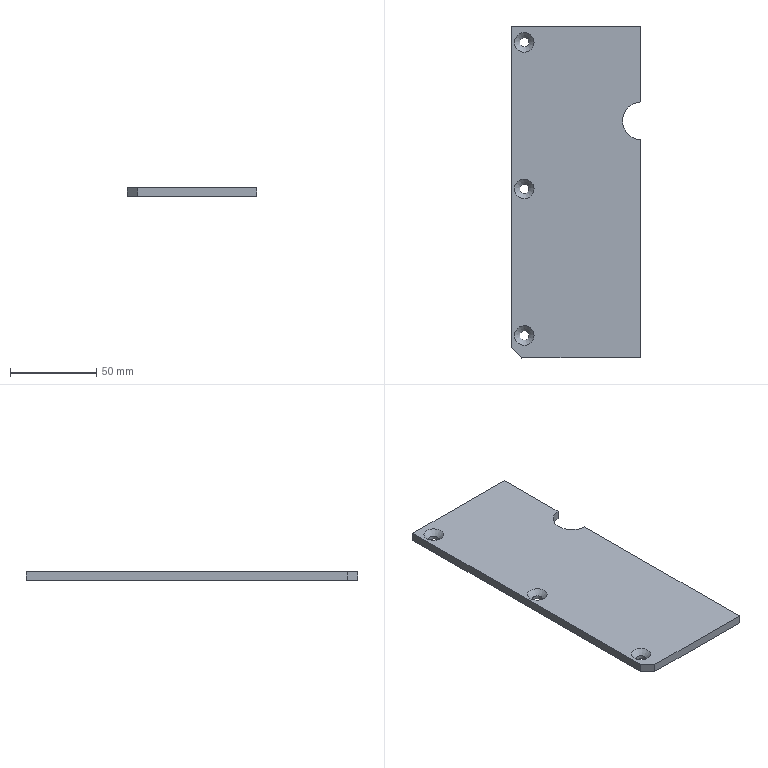Part | STEP file | P011002NF05-000 | 1 solid | 15 faces | box 75 x 192.5 x 5 mm | volume 70540 mm3 | plane 8 | cylinder 4 | cone 3 | commonest cylinder face diameters 5.5 x3 22 x1
STEP:
#1=CARTESIAN_POINT('',(0.,0.,0.));
#2=DIRECTION('',(0.,0.,1.));
#3=DIRECTION('',(1.,0.,0.));
#4=AXIS2_PLACEMENT_3D('',#1,#2,#3);
#5=CARTESIAN_POINT('',(-200.,233.25,265.5));
#6=VERTEX_POINT('',#5);
#7=CARTESIAN_POINT('',(-200.,230.5,265.5));
#8=DIRECTION('',(0.,0.,1.));
#9=DIRECTION('',(0.,1.,0.));
#10=AXIS2_PLACEMENT_3D('',#7,#8,#9);
#11=CIRCLE('',#10,2.75);
#12=CARTESIAN_POINT('',(-80.,170.,265.5));
#13=DIRECTION('',(0.,0.,-1.));
#14=DIRECTION('',(-1.,0.,0.));
#15=AXIS2_PLACEMENT_3D('',#12,#13,#14);
#16=PLANE('',#15);
#17=CARTESIAN_POINT('',(120.,63.25));
#18=CARTESIAN_POINT('',(124.763,63.25));
#19=CARTESIAN_POINT('',(122.382,59.125));
#20=CARTESIAN_POINT('',(120.,55.));
#21=CARTESIAN_POINT('',(117.618,59.125));
#22=CARTESIAN_POINT('',(115.237,63.25));
#23=CARTESIAN_POINT('',(120.,63.25));
#24=(BOUNDED_CURVE()B_SPLINE_CURVE(2,(#17,#18,#19,#20,#21,#22,#23),.UNSPECIFIED.,.T.,.F.)B_SPLINE_CURVE_WITH_KNOTS((1,2,2,2,2,1),(-2.094,0.,2.094,4.189,6.283,8.378),.UNSPECIFIED.)CURVE()GEOMETRIC_REPRESENTATION_ITEM()RATIONAL_B_SPLINE_CURVE((1.,0.5,1.,0.5,1.,0.5,1.))REPRESENTATION_ITEM(''));
#25=(GEOMETRIC_REPRESENTATION_CONTEXT(2)PARAMETRIC_REPRESENTATION_CONTEXT()REPRESENTATION_CONTEXT('',''));
#26=DEFINITIONAL_REPRESENTATION('',(#24),#25);
#27=PCURVE('',#16,#26);
#28=CARTESIAN_POINT('',(-200.,230.5,267.3));
#29=DIRECTION('',(0.,0.,-1.));
#30=DIRECTION('',(0.,1.,0.));
#31=AXIS2_PLACEMENT_3D('',#28,#29,#30);
#32=CYLINDRICAL_SURFACE('',#31,2.75);
#33=CARTESIAN_POINT('',(6.283,1.8));
#34=DIRECTION('',(-1.,0.));
#35=VECTOR('',#34,1.);
#36=LINE('',#33,#35);
#37=(GEOMETRIC_REPRESENTATION_CONTEXT(2)PARAMETRIC_REPRESENTATION_CONTEXT()REPRESENTATION_CONTEXT('',''));
#38=DEFINITIONAL_REPRESENTATION('',(#36),#37);
#39=PCURVE('',#32,#38);
#40=SURFACE_CURVE('',#11,(#27,#39),.PCURVE_S1.);
#41=EDGE_CURVE('',#6,#6,#40,.T.);
#42=ORIENTED_EDGE('',*,*,#41,.T.);
#43=EDGE_LOOP('',(#42));
#44=FACE_BOUND('',#43,.T.);
#45=CARTESIAN_POINT('',(-201.5,132.5,265.5));
#46=VERTEX_POINT('',#45);
#47=CARTESIAN_POINT('',(-132.5,132.5,265.5));
#48=VERTEX_POINT('',#47);
#49=CARTESIAN_POINT('',(-85.5,132.5,265.5));
#50=DIRECTION('',(1.,0.,0.));
#51=VECTOR('',#50,1.);
#52=LINE('',#49,#51);
#53=CARTESIAN_POINT('',(5.5,-37.5));
#54=DIRECTION('',(-1.,0.));
#55=VECTOR('',#54,1.);
#56=LINE('',#53,#55);
#57=(GEOMETRIC_REPRESENTATION_CONTEXT(2)PARAMETRIC_REPRESENTATION_CONTEXT()REPRESENTATION_CONTEXT('',''));
#58=DEFINITIONAL_REPRESENTATION('',(#56),#57);
#59=PCURVE('',#16,#58);
#60=CARTESIAN_POINT('',(-85.5,132.5,271.));
#61=DIRECTION('',(0.,-1.,0.));
#62=DIRECTION('',(1.,0.,0.));
#63=AXIS2_PLACEMENT_3D('',#60,#61,#62);
#64=PLANE('',#63);
#65=CARTESIAN_POINT('',(0.,-5.5));
#66=DIRECTION('',(1.,0.));
#67=VECTOR('',#66,1.);
#68=LINE('',#65,#67);
#69=(GEOMETRIC_REPRESENTATION_CONTEXT(2)PARAMETRIC_REPRESENTATION_CONTEXT()REPRESENTATION_CONTEXT('',''));
#70=DEFINITIONAL_REPRESENTATION('',(#68),#69);
#71=PCURVE('',#64,#70);
#72=SURFACE_CURVE('',#52,(#59,#71),.PCURVE_S1.);
#73=EDGE_CURVE('',#46,#48,#72,.T.);
#74=ORIENTED_EDGE('',*,*,#73,.F.);
#75=CARTESIAN_POINT('',(-207.5,138.5,265.5));
#76=VERTEX_POINT('',#75);
#77=CARTESIAN_POINT('',(-159.5,90.5,265.5));
#78=DIRECTION('',(-0.7071,0.7071,0.));
#79=VECTOR('',#78,1.);
#80=LINE('',#77,#79);
#81=CARTESIAN_POINT('',(79.5,-79.5));
#82=DIRECTION('',(0.7071,0.7071));
#83=VECTOR('',#82,1.);
#84=LINE('',#81,#83);
#85=(GEOMETRIC_REPRESENTATION_CONTEXT(2)PARAMETRIC_REPRESENTATION_CONTEXT()REPRESENTATION_CONTEXT('',''));
#86=DEFINITIONAL_REPRESENTATION('',(#84),#85);
#87=PCURVE('',#16,#86);
#88=CARTESIAN_POINT('',(-207.5,138.5,264.5));
#89=DIRECTION('',(0.7071,0.7071,0.));
#90=DIRECTION('',(-0.7071,0.7071,0.));
#91=AXIS2_PLACEMENT_3D('',#88,#89,#90);
#92=PLANE('',#91);
#93=CARTESIAN_POINT('',(-67.882,1.));
#94=DIRECTION('',(1.,0.));
#95=VECTOR('',#94,1.);
#96=LINE('',#93,#95);
#97=(GEOMETRIC_REPRESENTATION_CONTEXT(2)PARAMETRIC_REPRESENTATION_CONTEXT()REPRESENTATION_CONTEXT('',''));
#98=DEFINITIONAL_REPRESENTATION('',(#96),#97);
#99=PCURVE('',#92,#98);
#100=SURFACE_CURVE('',#80,(#87,#99),.PCURVE_S1.);
#101=EDGE_CURVE('',#46,#76,#100,.T.);
#102=ORIENTED_EDGE('',*,*,#101,.T.);
#103=CARTESIAN_POINT('',(-207.5,325.,265.5));
#104=VERTEX_POINT('',#103);
#105=CARTESIAN_POINT('',(-207.5,295.,265.5));
#106=DIRECTION('',(0.,-1.,0.));
#107=VECTOR('',#106,1.);
#108=LINE('',#105,#107);
#109=CARTESIAN_POINT('',(127.5,125.));
#110=DIRECTION('',(0.,-1.));
#111=VECTOR('',#110,1.);
#112=LINE('',#109,#111);
#113=(GEOMETRIC_REPRESENTATION_CONTEXT(2)PARAMETRIC_REPRESENTATION_CONTEXT()REPRESENTATION_CONTEXT('',''));
#114=DEFINITIONAL_REPRESENTATION('',(#112),#113);
#115=PCURVE('',#16,#114);
#116=CARTESIAN_POINT('',(-207.5,295.,264.5));
#117=DIRECTION('',(-1.,0.,0.));
#118=DIRECTION('',(0.,0.,1.));
#119=AXIS2_PLACEMENT_3D('',#116,#117,#118);
#120=PLANE('',#119);
#121=CARTESIAN_POINT('',(1.,0.));
#122=DIRECTION('',(0.,-1.));
#123=VECTOR('',#122,1.);
#124=LINE('',#121,#123);
#125=(GEOMETRIC_REPRESENTATION_CONTEXT(2)PARAMETRIC_REPRESENTATION_CONTEXT()REPRESENTATION_CONTEXT('',''));
#126=DEFINITIONAL_REPRESENTATION('',(#124),#125);
#127=PCURVE('',#120,#126);
#128=SURFACE_CURVE('',#108,(#115,#127),.PCURVE_S1.);
#129=EDGE_CURVE('',#104,#76,#128,.T.);
#130=ORIENTED_EDGE('',*,*,#129,.F.);
#131=CARTESIAN_POINT('',(-132.5,325.,265.5));
#132=VERTEX_POINT('',#131);
#133=CARTESIAN_POINT('',(-325.,325.,265.5));
#134=DIRECTION('',(-1.,0.,0.));
#135=VECTOR('',#134,1.);
#136=LINE('',#133,#135);
#137=CARTESIAN_POINT('',(245.,155.));
#138=DIRECTION('',(1.,0.));
#139=VECTOR('',#138,1.);
#140=LINE('',#137,#139);
#141=(GEOMETRIC_REPRESENTATION_CONTEXT(2)PARAMETRIC_REPRESENTATION_CONTEXT()REPRESENTATION_CONTEXT('',''));
#142=DEFINITIONAL_REPRESENTATION('',(#140),#141);
#143=PCURVE('',#16,#142);
#144=CARTESIAN_POINT('',(-325.,325.,260.));
#145=DIRECTION('',(0.,1.,0.));
#146=DIRECTION('',(0.,0.,1.));
#147=AXIS2_PLACEMENT_3D('',#144,#145,#146);
#148=PLANE('',#147);
#149=CARTESIAN_POINT('',(5.5,0.));
#150=DIRECTION('',(0.,-1.));
#151=VECTOR('',#150,1.);
#152=LINE('',#149,#151);
#153=(GEOMETRIC_REPRESENTATION_CONTEXT(2)PARAMETRIC_REPRESENTATION_CONTEXT()REPRESENTATION_CONTEXT('',''));
#154=DEFINITIONAL_REPRESENTATION('',(#152),#153);
#155=PCURVE('',#148,#154);
#156=SURFACE_CURVE('',#136,(#143,#155),.PCURVE_S1.);
#157=EDGE_CURVE('',#132,#104,#156,.T.);
#158=ORIENTED_EDGE('',*,*,#157,.F.);
#159=CARTESIAN_POINT('',(-132.5,280.989,265.5));
#160=VERTEX_POINT('',#159);
#161=CARTESIAN_POINT('',(-132.5,295.,265.5));
#162=DIRECTION('',(0.,1.,0.));
#163=VECTOR('',#162,1.);
#164=LINE('',#161,#163);
#165=CARTESIAN_POINT('',(52.5,125.));
#166=DIRECTION('',(0.,1.));
#167=VECTOR('',#166,1.);
#168=LINE('',#165,#167);
#169=(GEOMETRIC_REPRESENTATION_CONTEXT(2)PARAMETRIC_REPRESENTATION_CONTEXT()REPRESENTATION_CONTEXT('',''));
#170=DEFINITIONAL_REPRESENTATION('',(#168),#169);
#171=PCURVE('',#16,#170);
#172=CARTESIAN_POINT('',(-132.5,295.,264.5));
#173=DIRECTION('',(1.,0.,0.));
#174=DIRECTION('',(0.,0.,-1.));
#175=AXIS2_PLACEMENT_3D('',#172,#173,#174);
#176=PLANE('',#175);
#177=CARTESIAN_POINT('',(-1.,0.));
#178=DIRECTION('',(0.,1.));
#179=VECTOR('',#178,1.);
#180=LINE('',#177,#179);
#181=(GEOMETRIC_REPRESENTATION_CONTEXT(2)PARAMETRIC_REPRESENTATION_CONTEXT()REPRESENTATION_CONTEXT('',''));
#182=DEFINITIONAL_REPRESENTATION('',(#180),#181);
#183=PCURVE('',#176,#182);
#184=SURFACE_CURVE('',#164,(#171,#183),.PCURVE_S1.);
#185=EDGE_CURVE('',#160,#132,#184,.T.);
#186=ORIENTED_EDGE('',*,*,#185,.F.);
#187=CARTESIAN_POINT('',(-132.5,259.011,265.5));
#188=VERTEX_POINT('',#187);
#189=CARTESIAN_POINT('',(-132.,270.,265.5));
#190=DIRECTION('',(0.,0.,-1.));
#191=DIRECTION('',(-1.,0.,0.));
#192=AXIS2_PLACEMENT_3D('',#189,#190,#191);
#193=CIRCLE('',#192,11.);
#194=CARTESIAN_POINT('',(52.,100.));
#195=DIRECTION('',(1.,0.));
#196=AXIS2_PLACEMENT_2D('',#194,#195);
#197=CIRCLE('',#196,11.);
#198=(GEOMETRIC_REPRESENTATION_CONTEXT(2)PARAMETRIC_REPRESENTATION_CONTEXT()REPRESENTATION_CONTEXT('',''));
#199=DEFINITIONAL_REPRESENTATION('',(#197),#198);
#200=PCURVE('',#16,#199);
#201=CARTESIAN_POINT('',(-132.,270.,291.));
#202=DIRECTION('',(0.,0.,-1.));
#203=DIRECTION('',(-1.,0.,0.));
#204=AXIS2_PLACEMENT_3D('',#201,#202,#203);
#205=CYLINDRICAL_SURFACE('',#204,11.);
#206=CARTESIAN_POINT('',(-6.283,25.5));
#207=DIRECTION('',(1.,0.));
#208=VECTOR('',#207,1.);
#209=LINE('',#206,#208);
#210=(GEOMETRIC_REPRESENTATION_CONTEXT(2)PARAMETRIC_REPRESENTATION_CONTEXT()REPRESENTATION_CONTEXT('',''));
#211=DEFINITIONAL_REPRESENTATION('',(#209),#210);
#212=PCURVE('',#205,#211);
#213=SURFACE_CURVE('',#193,(#200,#212),.PCURVE_S1.);
#214=EDGE_CURVE('',#188,#160,#213,.T.);
#215=ORIENTED_EDGE('',*,*,#214,.F.);
#216=CARTESIAN_POINT('',(-132.5,295.,265.5));
#217=DIRECTION('',(0.,1.,0.));
#218=VECTOR('',#217,1.);
#219=LINE('',#216,#218);
#220=CARTESIAN_POINT('',(52.5,125.));
#221=DIRECTION('',(0.,1.));
#222=VECTOR('',#221,1.);
#223=LINE('',#220,#222);
#224=(GEOMETRIC_REPRESENTATION_CONTEXT(2)PARAMETRIC_REPRESENTATION_CONTEXT()REPRESENTATION_CONTEXT('',''));
#225=DEFINITIONAL_REPRESENTATION('',(#223),#224);
#226=PCURVE('',#16,#225);
#227=CARTESIAN_POINT('',(-132.5,295.,264.5));
#228=DIRECTION('',(1.,0.,0.));
#229=DIRECTION('',(0.,0.,-1.));
#230=AXIS2_PLACEMENT_3D('',#227,#228,#229);
#231=PLANE('',#230);
#232=CARTESIAN_POINT('',(-1.,0.));
#233=DIRECTION('',(0.,1.));
#234=VECTOR('',#233,1.);
#235=LINE('',#232,#234);
#236=(GEOMETRIC_REPRESENTATION_CONTEXT(2)PARAMETRIC_REPRESENTATION_CONTEXT()REPRESENTATION_CONTEXT('',''));
#237=DEFINITIONAL_REPRESENTATION('',(#235),#236);
#238=PCURVE('',#231,#237);
#239=SURFACE_CURVE('',#219,(#226,#238),.PCURVE_S1.);
#240=EDGE_CURVE('',#48,#188,#239,.T.);
#241=ORIENTED_EDGE('',*,*,#240,.F.);
#242=EDGE_LOOP('',(#74,#102,#130,#158,#186,#215,#241));
#243=FACE_BOUND('',#242,.T.);
#244=CARTESIAN_POINT('',(-200.,148.25,265.5));
#245=VERTEX_POINT('',#244);
#246=CARTESIAN_POINT('',(-200.,145.5,265.5));
#247=DIRECTION('',(0.,0.,1.));
#248=DIRECTION('',(0.,1.,0.));
#249=AXIS2_PLACEMENT_3D('',#246,#247,#248);
#250=CIRCLE('',#249,2.75);
#251=CARTESIAN_POINT('',(120.,-21.75));
#252=CARTESIAN_POINT('',(124.763,-21.75));
#253=CARTESIAN_POINT('',(122.382,-25.875));
#254=CARTESIAN_POINT('',(120.,-30.));
#255=CARTESIAN_POINT('',(117.618,-25.875));
#256=CARTESIAN_POINT('',(115.237,-21.75));
#257=CARTESIAN_POINT('',(120.,-21.75));
#258=(BOUNDED_CURVE()B_SPLINE_CURVE(2,(#251,#252,#253,#254,#255,#256,#257),.UNSPECIFIED.,.T.,.F.)B_SPLINE_CURVE_WITH_KNOTS((1,2,2,2,2,1),(-2.094,0.,2.094,4.189,6.283,8.378),.UNSPECIFIED.)CURVE()GEOMETRIC_REPRESENTATION_ITEM()RATIONAL_B_SPLINE_CURVE((1.,0.5,1.,0.5,1.,0.5,1.))REPRESENTATION_ITEM(''));
#259=(GEOMETRIC_REPRESENTATION_CONTEXT(2)PARAMETRIC_REPRESENTATION_CONTEXT()REPRESENTATION_CONTEXT('',''));
#260=DEFINITIONAL_REPRESENTATION('',(#258),#259);
#261=PCURVE('',#16,#260);
#262=CARTESIAN_POINT('',(-200.,145.5,267.3));
#263=DIRECTION('',(0.,0.,-1.));
#264=DIRECTION('',(0.,1.,0.));
#265=AXIS2_PLACEMENT_3D('',#262,#263,#264);
#266=CYLINDRICAL_SURFACE('',#265,2.75);
#267=CARTESIAN_POINT('',(6.283,1.8));
#268=DIRECTION('',(-1.,0.));
#269=VECTOR('',#268,1.);
#270=LINE('',#267,#269);
#271=(GEOMETRIC_REPRESENTATION_CONTEXT(2)PARAMETRIC_REPRESENTATION_CONTEXT()REPRESENTATION_CONTEXT('',''));
#272=DEFINITIONAL_REPRESENTATION('',(#270),#271);
#273=PCURVE('',#266,#272);
#274=SURFACE_CURVE('',#250,(#261,#273),.PCURVE_S1.);
#275=EDGE_CURVE('',#245,#245,#274,.T.);
#276=ORIENTED_EDGE('',*,*,#275,.T.);
#277=EDGE_LOOP('',(#276));
#278=FACE_BOUND('',#277,.T.);
#279=CARTESIAN_POINT('',(-200.,318.25,265.5));
#280=VERTEX_POINT('',#279);
#281=CARTESIAN_POINT('',(-200.,315.5,265.5));
#282=DIRECTION('',(0.,0.,1.));
#283=DIRECTION('',(0.,1.,0.));
#284=AXIS2_PLACEMENT_3D('',#281,#282,#283);
#285=CIRCLE('',#284,2.75);
#286=CARTESIAN_POINT('',(120.,148.25));
#287=CARTESIAN_POINT('',(124.763,148.25));
#288=CARTESIAN_POINT('',(122.382,144.125));
#289=CARTESIAN_POINT('',(120.,140.));
#290=CARTESIAN_POINT('',(117.618,144.125));
#291=CARTESIAN_POINT('',(115.237,148.25));
#292=CARTESIAN_POINT('',(120.,148.25));
#293=(BOUNDED_CURVE()B_SPLINE_CURVE(2,(#286,#287,#288,#289,#290,#291,#292),.UNSPECIFIED.,.T.,.F.)B_SPLINE_CURVE_WITH_KNOTS((1,2,2,2,2,1),(-2.094,0.,2.094,4.189,6.283,8.378),.UNSPECIFIED.)CURVE()GEOMETRIC_REPRESENTATION_ITEM()RATIONAL_B_SPLINE_CURVE((1.,0.5,1.,0.5,1.,0.5,1.))REPRESENTATION_ITEM(''));
#294=(GEOMETRIC_REPRESENTATION_CONTEXT(2)PARAMETRIC_REPRESENTATION_CONTEXT()REPRESENTATION_CONTEXT('',''));
#295=DEFINITIONAL_REPRESENTATION('',(#293),#294);
#296=PCURVE('',#16,#295);
#297=CARTESIAN_POINT('',(-200.,315.5,267.3));
#298=DIRECTION('',(0.,0.,-1.));
#299=DIRECTION('',(0.,1.,0.));
#300=AXIS2_PLACEMENT_3D('',#297,#298,#299);
#301=CYLINDRICAL_SURFACE('',#300,2.75);
#302=CARTESIAN_POINT('',(6.283,1.8));
#303=DIRECTION('',(-1.,0.));
#304=VECTOR('',#303,1.);
#305=LINE('',#302,#304);
#306=(GEOMETRIC_REPRESENTATION_CONTEXT(2)PARAMETRIC_REPRESENTATION_CONTEXT()REPRESENTATION_CONTEXT('',''));
#307=DEFINITIONAL_REPRESENTATION('',(#305),#306);
#308=PCURVE('',#301,#307);
#309=SURFACE_CURVE('',#285,(#296,#308),.PCURVE_S1.);
#310=EDGE_CURVE('',#280,#280,#309,.T.);
#311=ORIENTED_EDGE('',*,*,#310,.T.);
#312=EDGE_LOOP('',(#311));
#313=FACE_BOUND('',#312,.T.);
#314=ADVANCED_FACE('',(#44,#243,#278,#313),#16,.T.);
#315=CARTESIAN_POINT('',(-132.5,259.011,270.5));
#316=VERTEX_POINT('',#315);
#317=CARTESIAN_POINT('',(-132.5,259.011,291.));
#318=DIRECTION('',(0.,0.,-1.));
#319=VECTOR('',#318,1.);
#320=LINE('',#317,#319);
#321=CARTESIAN_POINT('',(-26.5,-35.989));
#322=DIRECTION('',(1.,0.));
#323=VECTOR('',#322,1.);
#324=LINE('',#321,#323);
#325=(GEOMETRIC_REPRESENTATION_CONTEXT(2)PARAMETRIC_REPRESENTATION_CONTEXT()REPRESENTATION_CONTEXT('',''));
#326=DEFINITIONAL_REPRESENTATION('',(#324),#325);
#327=PCURVE('',#231,#326);
#328=CARTESIAN_POINT('',(-1.525,0.));
#329=DIRECTION('',(0.,1.));
#330=VECTOR('',#329,1.);
#331=LINE('',#328,#330);
#332=(GEOMETRIC_REPRESENTATION_CONTEXT(2)PARAMETRIC_REPRESENTATION_CONTEXT()REPRESENTATION_CONTEXT('',''));
#333=DEFINITIONAL_REPRESENTATION('',(#331),#332);
#334=PCURVE('',#205,#333);
#335=SURFACE_CURVE('',#320,(#327,#334),.PCURVE_S1.);
#336=EDGE_CURVE('',#316,#188,#335,.T.);
#337=ORIENTED_EDGE('',*,*,#336,.F.);
#338=CARTESIAN_POINT('',(-132.5,132.5,270.5));
#339=VERTEX_POINT('',#338);
#340=CARTESIAN_POINT('',(-132.5,295.,270.5));
#341=DIRECTION('',(0.,-1.,0.));
#342=VECTOR('',#341,1.);
#343=LINE('',#340,#342);
#344=CARTESIAN_POINT('',(-6.,0.));
#345=DIRECTION('',(0.,-1.));
#346=VECTOR('',#345,1.);
#347=LINE('',#344,#346);
#348=(GEOMETRIC_REPRESENTATION_CONTEXT(2)PARAMETRIC_REPRESENTATION_CONTEXT()REPRESENTATION_CONTEXT('',''));
#349=DEFINITIONAL_REPRESENTATION('',(#347),#348);
#350=PCURVE('',#231,#349);
#351=CARTESIAN_POINT('',(275.,325.,270.5));
#352=DIRECTION('',(0.,0.,-1.));
#353=DIRECTION('',(-1.,0.,0.));
#354=AXIS2_PLACEMENT_3D('',#351,#352,#353);
#355=PLANE('',#354);
#356=CARTESIAN_POINT('',(407.5,-30.));
#357=DIRECTION('',(0.,-1.));
#358=VECTOR('',#357,1.);
#359=LINE('',#356,#358);
#360=(GEOMETRIC_REPRESENTATION_CONTEXT(2)PARAMETRIC_REPRESENTATION_CONTEXT()REPRESENTATION_CONTEXT('',''));
#361=DEFINITIONAL_REPRESENTATION('',(#359),#360);
#362=PCURVE('',#355,#361);
#363=SURFACE_CURVE('',#343,(#350,#362),.PCURVE_S1.);
#364=EDGE_CURVE('',#316,#339,#363,.T.);
#365=ORIENTED_EDGE('',*,*,#364,.T.);
#366=CARTESIAN_POINT('',(-132.5,132.5,271.));
#367=DIRECTION('',(0.,0.,1.));
#368=VECTOR('',#367,1.);
#369=LINE('',#366,#368);
#370=CARTESIAN_POINT('',(-6.5,-162.5));
#371=DIRECTION('',(-1.,0.));
#372=VECTOR('',#371,1.);
#373=LINE('',#370,#372);
#374=(GEOMETRIC_REPRESENTATION_CONTEXT(2)PARAMETRIC_REPRESENTATION_CONTEXT()REPRESENTATION_CONTEXT('',''));
#375=DEFINITIONAL_REPRESENTATION('',(#373),#374);
#376=PCURVE('',#231,#375);
#377=CARTESIAN_POINT('',(-47.,0.));
#378=DIRECTION('',(0.,1.));
#379=VECTOR('',#378,1.);
#380=LINE('',#377,#379);
#381=(GEOMETRIC_REPRESENTATION_CONTEXT(2)PARAMETRIC_REPRESENTATION_CONTEXT()REPRESENTATION_CONTEXT('',''));
#382=DEFINITIONAL_REPRESENTATION('',(#380),#381);
#383=PCURVE('',#64,#382);
#384=SURFACE_CURVE('',#369,(#376,#383),.PCURVE_S1.);
#385=EDGE_CURVE('',#48,#339,#384,.T.);
#386=ORIENTED_EDGE('',*,*,#385,.F.);
#387=ORIENTED_EDGE('',*,*,#240,.T.);
#388=EDGE_LOOP('',(#337,#365,#386,#387));
#389=FACE_BOUND('',#388,.T.);
#390=ADVANCED_FACE('',(#389),#231,.T.);
#391=CARTESIAN_POINT('',(-194.3,315.5,270.5));
#392=VERTEX_POINT('',#391);
#393=CARTESIAN_POINT('',(-200.,321.2,270.5));
#394=VERTEX_POINT('',#393);
#395=CARTESIAN_POINT('',(-200.,315.5,270.5));
#396=DIRECTION('',(0.,0.,1.));
#397=DIRECTION('',(1.,0.,0.));
#398=AXIS2_PLACEMENT_3D('',#395,#396,#397);
#399=CIRCLE('',#398,5.7);
#400=CARTESIAN_POINT('',(469.3,-9.5));
#401=CARTESIAN_POINT('',(469.3,0.3727));
#402=CARTESIAN_POINT('',(477.85,-4.564));
#403=CARTESIAN_POINT('',(486.4,-9.5));
#404=CARTESIAN_POINT('',(477.85,-14.436));
#405=CARTESIAN_POINT('',(469.3,-19.373));
#406=CARTESIAN_POINT('',(469.3,-9.5));
#407=(BOUNDED_CURVE()B_SPLINE_CURVE(2,(#400,#401,#402,#403,#404,#405,#406),.UNSPECIFIED.,.T.,.F.)B_SPLINE_CURVE_WITH_KNOTS((1,2,2,2,2,1),(-2.094,0.,2.094,4.189,6.283,8.378),.UNSPECIFIED.)CURVE()GEOMETRIC_REPRESENTATION_ITEM()RATIONAL_B_SPLINE_CURVE((1.,0.5,1.,0.5,1.,0.5,1.))REPRESENTATION_ITEM(''));
#408=(GEOMETRIC_REPRESENTATION_CONTEXT(2)PARAMETRIC_REPRESENTATION_CONTEXT()REPRESENTATION_CONTEXT('',''));
#409=DEFINITIONAL_REPRESENTATION('',(#407),#408);
#410=PCURVE('',#355,#409);
#411=CARTESIAN_POINT('',(-200.,315.5,267.3));
#412=DIRECTION('',(0.,0.,1.));
#413=DIRECTION('',(0.,1.,0.));
#414=AXIS2_PLACEMENT_3D('',#411,#412,#413);
#415=CONICAL_SURFACE('',#414,2.5,0.7854);
#416=CARTESIAN_POINT('',(4.712,3.2));
#417=DIRECTION('',(1.,0.));
#418=VECTOR('',#417,1.);
#419=LINE('',#416,#418);
#420=(GEOMETRIC_REPRESENTATION_CONTEXT(2)PARAMETRIC_REPRESENTATION_CONTEXT()REPRESENTATION_CONTEXT('',''));
#421=DEFINITIONAL_REPRESENTATION('',(#419),#420);
#422=PCURVE('',#415,#421);
#423=SURFACE_CURVE('',#399,(#410,#422),.PCURVE_S1.);
#424=EDGE_CURVE('',#392,#394,#423,.T.);
#425=ORIENTED_EDGE('',*,*,#424,.F.);
#426=CARTESIAN_POINT('',(-200.,315.5,270.5));
#427=DIRECTION('',(0.,0.,1.));
#428=DIRECTION('',(1.,0.,0.));
#429=AXIS2_PLACEMENT_3D('',#426,#427,#428);
#430=CIRCLE('',#429,5.7);
#431=CARTESIAN_POINT('',(469.3,-9.5));
#432=CARTESIAN_POINT('',(469.3,0.3727));
#433=CARTESIAN_POINT('',(477.85,-4.564));
#434=CARTESIAN_POINT('',(486.4,-9.5));
#435=CARTESIAN_POINT('',(477.85,-14.436));
#436=CARTESIAN_POINT('',(469.3,-19.373));
#437=CARTESIAN_POINT('',(469.3,-9.5));
#438=(BOUNDED_CURVE()B_SPLINE_CURVE(2,(#431,#432,#433,#434,#435,#436,#437),.UNSPECIFIED.,.T.,.F.)B_SPLINE_CURVE_WITH_KNOTS((1,2,2,2,2,1),(-2.094,0.,2.094,4.189,6.283,8.378),.UNSPECIFIED.)CURVE()GEOMETRIC_REPRESENTATION_ITEM()RATIONAL_B_SPLINE_CURVE((1.,0.5,1.,0.5,1.,0.5,1.))REPRESENTATION_ITEM(''));
#439=(GEOMETRIC_REPRESENTATION_CONTEXT(2)PARAMETRIC_REPRESENTATION_CONTEXT()REPRESENTATION_CONTEXT('',''));
#440=DEFINITIONAL_REPRESENTATION('',(#438),#439);
#441=PCURVE('',#355,#440);
#442=CARTESIAN_POINT('',(-1.571,3.2));
#443=DIRECTION('',(1.,0.));
#444=VECTOR('',#443,1.);
#445=LINE('',#442,#444);
#446=(GEOMETRIC_REPRESENTATION_CONTEXT(2)PARAMETRIC_REPRESENTATION_CONTEXT()REPRESENTATION_CONTEXT('',''));
#447=DEFINITIONAL_REPRESENTATION('',(#445),#446);
#448=PCURVE('',#415,#447);
#449=SURFACE_CURVE('',#430,(#441,#448),.PCURVE_S1.);
#450=EDGE_CURVE('',#394,#392,#449,.T.);
#451=ORIENTED_EDGE('',*,*,#450,.F.);
#452=EDGE_LOOP('',(#425,#451));
#453=FACE_BOUND('',#452,.T.);
#454=CARTESIAN_POINT('',(-194.3,230.5,270.5));
#455=VERTEX_POINT('',#454);
#456=CARTESIAN_POINT('',(-200.,236.2,270.5));
#457=VERTEX_POINT('',#456);
#458=CARTESIAN_POINT('',(-200.,230.5,270.5));
#459=DIRECTION('',(0.,0.,1.));
#460=DIRECTION('',(1.,0.,0.));
#461=AXIS2_PLACEMENT_3D('',#458,#459,#460);
#462=CIRCLE('',#461,5.7);
#463=CARTESIAN_POINT('',(469.3,-94.5));
#464=CARTESIAN_POINT('',(469.3,-84.627));
#465=CARTESIAN_POINT('',(477.85,-89.564));
#466=CARTESIAN_POINT('',(486.4,-94.5));
#467=CARTESIAN_POINT('',(477.85,-99.436));
#468=CARTESIAN_POINT('',(469.3,-104.373));
#469=CARTESIAN_POINT('',(469.3,-94.5));
#470=(BOUNDED_CURVE()B_SPLINE_CURVE(2,(#463,#464,#465,#466,#467,#468,#469),.UNSPECIFIED.,.T.,.F.)B_SPLINE_CURVE_WITH_KNOTS((1,2,2,2,2,1),(-2.094,0.,2.094,4.189,6.283,8.378),.UNSPECIFIED.)CURVE()GEOMETRIC_REPRESENTATION_ITEM()RATIONAL_B_SPLINE_CURVE((1.,0.5,1.,0.5,1.,0.5,1.))REPRESENTATION_ITEM(''));
#471=(GEOMETRIC_REPRESENTATION_CONTEXT(2)PARAMETRIC_REPRESENTATION_CONTEXT()REPRESENTATION_CONTEXT('',''));
#472=DEFINITIONAL_REPRESENTATION('',(#470),#471);
#473=PCURVE('',#355,#472);
#474=CARTESIAN_POINT('',(-200.,230.5,267.3));
#475=DIRECTION('',(0.,0.,1.));
#476=DIRECTION('',(0.,1.,0.));
#477=AXIS2_PLACEMENT_3D('',#474,#475,#476);
#478=CONICAL_SURFACE('',#477,2.5,0.7854);
#479=CARTESIAN_POINT('',(4.712,3.2));
#480=DIRECTION('',(1.,0.));
#481=VECTOR('',#480,1.);
#482=LINE('',#479,#481);
#483=(GEOMETRIC_REPRESENTATION_CONTEXT(2)PARAMETRIC_REPRESENTATION_CONTEXT()REPRESENTATION_CONTEXT('',''));
#484=DEFINITIONAL_REPRESENTATION('',(#482),#483);
#485=PCURVE('',#478,#484);
#486=SURFACE_CURVE('',#462,(#473,#485),.PCURVE_S1.);
#487=EDGE_CURVE('',#455,#457,#486,.T.);
#488=ORIENTED_EDGE('',*,*,#487,.F.);
#489=CARTESIAN_POINT('',(-200.,230.5,270.5));
#490=DIRECTION('',(0.,0.,1.));
#491=DIRECTION('',(1.,0.,0.));
#492=AXIS2_PLACEMENT_3D('',#489,#490,#491);
#493=CIRCLE('',#492,5.7);
#494=CARTESIAN_POINT('',(469.3,-94.5));
#495=CARTESIAN_POINT('',(469.3,-84.627));
#496=CARTESIAN_POINT('',(477.85,-89.564));
#497=CARTESIAN_POINT('',(486.4,-94.5));
#498=CARTESIAN_POINT('',(477.85,-99.436));
#499=CARTESIAN_POINT('',(469.3,-104.373));
#500=CARTESIAN_POINT('',(469.3,-94.5));
#501=(BOUNDED_CURVE()B_SPLINE_CURVE(2,(#494,#495,#496,#497,#498,#499,#500),.UNSPECIFIED.,.T.,.F.)B_SPLINE_CURVE_WITH_KNOTS((1,2,2,2,2,1),(-2.094,0.,2.094,4.189,6.283,8.378),.UNSPECIFIED.)CURVE()GEOMETRIC_REPRESENTATION_ITEM()RATIONAL_B_SPLINE_CURVE((1.,0.5,1.,0.5,1.,0.5,1.))REPRESENTATION_ITEM(''));
#502=(GEOMETRIC_REPRESENTATION_CONTEXT(2)PARAMETRIC_REPRESENTATION_CONTEXT()REPRESENTATION_CONTEXT('',''));
#503=DEFINITIONAL_REPRESENTATION('',(#501),#502);
#504=PCURVE('',#355,#503);
#505=CARTESIAN_POINT('',(-1.571,3.2));
#506=DIRECTION('',(1.,0.));
#507=VECTOR('',#506,1.);
#508=LINE('',#505,#507);
#509=(GEOMETRIC_REPRESENTATION_CONTEXT(2)PARAMETRIC_REPRESENTATION_CONTEXT()REPRESENTATION_CONTEXT('',''));
#510=DEFINITIONAL_REPRESENTATION('',(#508),#509);
#511=PCURVE('',#478,#510);
#512=SURFACE_CURVE('',#493,(#504,#511),.PCURVE_S1.);
#513=EDGE_CURVE('',#457,#455,#512,.T.);
#514=ORIENTED_EDGE('',*,*,#513,.F.);
#515=EDGE_LOOP('',(#488,#514));
#516=FACE_BOUND('',#515,.T.);
#517=CARTESIAN_POINT('',(-194.3,145.5,270.5));
#518=VERTEX_POINT('',#517);
#519=CARTESIAN_POINT('',(-200.,151.2,270.5));
#520=VERTEX_POINT('',#519);
#521=CARTESIAN_POINT('',(-200.,145.5,270.5));
#522=DIRECTION('',(0.,0.,1.));
#523=DIRECTION('',(1.,0.,0.));
#524=AXIS2_PLACEMENT_3D('',#521,#522,#523);
#525=CIRCLE('',#524,5.7);
#526=CARTESIAN_POINT('',(469.3,-179.5));
#527=CARTESIAN_POINT('',(469.3,-169.627));
#528=CARTESIAN_POINT('',(477.85,-174.564));
#529=CARTESIAN_POINT('',(486.4,-179.5));
#530=CARTESIAN_POINT('',(477.85,-184.436));
#531=CARTESIAN_POINT('',(469.3,-189.373));
#532=CARTESIAN_POINT('',(469.3,-179.5));
#533=(BOUNDED_CURVE()B_SPLINE_CURVE(2,(#526,#527,#528,#529,#530,#531,#532),.UNSPECIFIED.,.T.,.F.)B_SPLINE_CURVE_WITH_KNOTS((1,2,2,2,2,1),(-2.094,0.,2.094,4.189,6.283,8.378),.UNSPECIFIED.)CURVE()GEOMETRIC_REPRESENTATION_ITEM()RATIONAL_B_SPLINE_CURVE((1.,0.5,1.,0.5,1.,0.5,1.))REPRESENTATION_ITEM(''));
#534=(GEOMETRIC_REPRESENTATION_CONTEXT(2)PARAMETRIC_REPRESENTATION_CONTEXT()REPRESENTATION_CONTEXT('',''));
#535=DEFINITIONAL_REPRESENTATION('',(#533),#534);
#536=PCURVE('',#355,#535);
#537=CARTESIAN_POINT('',(-200.,145.5,267.3));
#538=DIRECTION('',(0.,0.,1.));
#539=DIRECTION('',(0.,1.,0.));
#540=AXIS2_PLACEMENT_3D('',#537,#538,#539);
#541=CONICAL_SURFACE('',#540,2.5,0.7854);
#542=CARTESIAN_POINT('',(4.712,3.2));
#543=DIRECTION('',(1.,0.));
#544=VECTOR('',#543,1.);
#545=LINE('',#542,#544);
#546=(GEOMETRIC_REPRESENTATION_CONTEXT(2)PARAMETRIC_REPRESENTATION_CONTEXT()REPRESENTATION_CONTEXT('',''));
#547=DEFINITIONAL_REPRESENTATION('',(#545),#546);
#548=PCURVE('',#541,#547);
#549=SURFACE_CURVE('',#525,(#536,#548),.PCURVE_S1.);
#550=EDGE_CURVE('',#518,#520,#549,.T.);
#551=ORIENTED_EDGE('',*,*,#550,.F.);
#552=CARTESIAN_POINT('',(-200.,145.5,270.5));
#553=DIRECTION('',(0.,0.,1.));
#554=DIRECTION('',(1.,0.,0.));
#555=AXIS2_PLACEMENT_3D('',#552,#553,#554);
#556=CIRCLE('',#555,5.7);
#557=CARTESIAN_POINT('',(469.3,-179.5));
#558=CARTESIAN_POINT('',(469.3,-169.627));
#559=CARTESIAN_POINT('',(477.85,-174.564));
#560=CARTESIAN_POINT('',(486.4,-179.5));
#561=CARTESIAN_POINT('',(477.85,-184.436));
#562=CARTESIAN_POINT('',(469.3,-189.373));
#563=CARTESIAN_POINT('',(469.3,-179.5));
#564=(BOUNDED_CURVE()B_SPLINE_CURVE(2,(#557,#558,#559,#560,#561,#562,#563),.UNSPECIFIED.,.T.,.F.)B_SPLINE_CURVE_WITH_KNOTS((1,2,2,2,2,1),(-2.094,0.,2.094,4.189,6.283,8.378),.UNSPECIFIED.)CURVE()GEOMETRIC_REPRESENTATION_ITEM()RATIONAL_B_SPLINE_CURVE((1.,0.5,1.,0.5,1.,0.5,1.))REPRESENTATION_ITEM(''));
#565=(GEOMETRIC_REPRESENTATION_CONTEXT(2)PARAMETRIC_REPRESENTATION_CONTEXT()REPRESENTATION_CONTEXT('',''));
#566=DEFINITIONAL_REPRESENTATION('',(#564),#565);
#567=PCURVE('',#355,#566);
#568=CARTESIAN_POINT('',(-1.571,3.2));
#569=DIRECTION('',(1.,0.));
#570=VECTOR('',#569,1.);
#571=LINE('',#568,#570);
#572=(GEOMETRIC_REPRESENTATION_CONTEXT(2)PARAMETRIC_REPRESENTATION_CONTEXT()REPRESENTATION_CONTEXT('',''));
#573=DEFINITIONAL_REPRESENTATION('',(#571),#572);
#574=PCURVE('',#541,#573);
#575=SURFACE_CURVE('',#556,(#567,#574),.PCURVE_S1.);
#576=EDGE_CURVE('',#520,#518,#575,.T.);
#577=ORIENTED_EDGE('',*,*,#576,.F.);
#578=EDGE_LOOP('',(#551,#577));
#579=FACE_BOUND('',#578,.T.);
#580=CARTESIAN_POINT('',(-207.5,138.5,270.5));
#581=VERTEX_POINT('',#580);
#582=CARTESIAN_POINT('',(-207.5,325.,270.5));
#583=VERTEX_POINT('',#582);
#584=CARTESIAN_POINT('',(-207.5,295.,270.5));
#585=DIRECTION('',(0.,1.,0.));
#586=VECTOR('',#585,1.);
#587=LINE('',#584,#586);
#588=CARTESIAN_POINT('',(482.5,-30.));
#589=DIRECTION('',(0.,1.));
#590=VECTOR('',#589,1.);
#591=LINE('',#588,#590);
#592=(GEOMETRIC_REPRESENTATION_CONTEXT(2)PARAMETRIC_REPRESENTATION_CONTEXT()REPRESENTATION_CONTEXT('',''));
#593=DEFINITIONAL_REPRESENTATION('',(#591),#592);
#594=PCURVE('',#355,#593);
#595=CARTESIAN_POINT('',(6.,0.));
#596=DIRECTION('',(0.,1.));
#597=VECTOR('',#596,1.);
#598=LINE('',#595,#597);
#599=(GEOMETRIC_REPRESENTATION_CONTEXT(2)PARAMETRIC_REPRESENTATION_CONTEXT()REPRESENTATION_CONTEXT('',''));
#600=DEFINITIONAL_REPRESENTATION('',(#598),#599);
#601=PCURVE('',#120,#600);
#602=SURFACE_CURVE('',#587,(#594,#601),.PCURVE_S1.);
#603=EDGE_CURVE('',#581,#583,#602,.T.);
#604=ORIENTED_EDGE('',*,*,#603,.F.);
#605=CARTESIAN_POINT('',(-201.5,132.5,270.5));
#606=VERTEX_POINT('',#605);
#607=CARTESIAN_POINT('',(-59.5,-9.5,270.5));
#608=DIRECTION('',(0.7071,-0.7071,0.));
#609=VECTOR('',#608,1.);
#610=LINE('',#607,#609);
#611=CARTESIAN_POINT('',(334.5,-334.5));
#612=DIRECTION('',(-0.7071,-0.7071));
#613=VECTOR('',#612,1.);
#614=LINE('',#611,#613);
#615=(GEOMETRIC_REPRESENTATION_CONTEXT(2)PARAMETRIC_REPRESENTATION_CONTEXT()REPRESENTATION_CONTEXT('',''));
#616=DEFINITIONAL_REPRESENTATION('',(#614),#615);
#617=PCURVE('',#355,#616);
#618=CARTESIAN_POINT('',(-209.304,6.));
#619=DIRECTION('',(-1.,0.));
#620=VECTOR('',#619,1.);
#621=LINE('',#618,#620);
#622=(GEOMETRIC_REPRESENTATION_CONTEXT(2)PARAMETRIC_REPRESENTATION_CONTEXT()REPRESENTATION_CONTEXT('',''));
#623=DEFINITIONAL_REPRESENTATION('',(#621),#622);
#624=PCURVE('',#92,#623);
#625=SURFACE_CURVE('',#610,(#617,#624),.PCURVE_S1.);
#626=EDGE_CURVE('',#581,#606,#625,.T.);
#627=ORIENTED_EDGE('',*,*,#626,.T.);
#628=CARTESIAN_POINT('',(-85.5,132.5,270.5));
#629=DIRECTION('',(-1.,0.,0.));
#630=VECTOR('',#629,1.);
#631=LINE('',#628,#630);
#632=CARTESIAN_POINT('',(360.5,-192.5));
#633=DIRECTION('',(1.,0.));
#634=VECTOR('',#633,1.);
#635=LINE('',#632,#634);
#636=(GEOMETRIC_REPRESENTATION_CONTEXT(2)PARAMETRIC_REPRESENTATION_CONTEXT()REPRESENTATION_CONTEXT('',''));
#637=DEFINITIONAL_REPRESENTATION('',(#635),#636);
#638=PCURVE('',#355,#637);
#639=CARTESIAN_POINT('',(0.,-0.5));
#640=DIRECTION('',(-1.,0.));
#641=VECTOR('',#640,1.);
#642=LINE('',#639,#641);
#643=(GEOMETRIC_REPRESENTATION_CONTEXT(2)PARAMETRIC_REPRESENTATION_CONTEXT()REPRESENTATION_CONTEXT('',''));
#644=DEFINITIONAL_REPRESENTATION('',(#642),#643);
#645=PCURVE('',#64,#644);
#646=SURFACE_CURVE('',#631,(#638,#645),.PCURVE_S1.);
#647=EDGE_CURVE('',#339,#606,#646,.T.);
#648=ORIENTED_EDGE('',*,*,#647,.F.);
#649=ORIENTED_EDGE('',*,*,#364,.F.);
#650=CARTESIAN_POINT('',(-132.5,280.989,270.5));
#651=VERTEX_POINT('',#650);
#652=CARTESIAN_POINT('',(-132.,270.,270.5));
#653=DIRECTION('',(0.,0.,1.));
#654=DIRECTION('',(-1.,0.,0.));
#655=AXIS2_PLACEMENT_3D('',#652,#653,#654);
#656=CIRCLE('',#655,11.);
#657=CARTESIAN_POINT('',(418.,-55.));
#658=CARTESIAN_POINT('',(418.,-74.053));
#659=CARTESIAN_POINT('',(401.5,-64.526));
#660=CARTESIAN_POINT('',(385.,-55.));
#661=CARTESIAN_POINT('',(401.5,-45.474));
#662=CARTESIAN_POINT('',(418.,-35.947));
#663=CARTESIAN_POINT('',(418.,-55.));
#664=(BOUNDED_CURVE()B_SPLINE_CURVE(2,(#657,#658,#659,#660,#661,#662,#663),.UNSPECIFIED.,.T.,.F.)B_SPLINE_CURVE_WITH_KNOTS((1,2,2,2,2,1),(-2.094,0.,2.094,4.189,6.283,8.378),.UNSPECIFIED.)CURVE()GEOMETRIC_REPRESENTATION_ITEM()RATIONAL_B_SPLINE_CURVE((1.,0.5,1.,0.5,1.,0.5,1.))REPRESENTATION_ITEM(''));
#665=(GEOMETRIC_REPRESENTATION_CONTEXT(2)PARAMETRIC_REPRESENTATION_CONTEXT()REPRESENTATION_CONTEXT('',''));
#666=DEFINITIONAL_REPRESENTATION('',(#664),#665);
#667=PCURVE('',#355,#666);
#668=CARTESIAN_POINT('',(6.283,20.5));
#669=DIRECTION('',(-1.,0.));
#670=VECTOR('',#669,1.);
#671=LINE('',#668,#670);
#672=(GEOMETRIC_REPRESENTATION_CONTEXT(2)PARAMETRIC_REPRESENTATION_CONTEXT()REPRESENTATION_CONTEXT('',''));
#673=DEFINITIONAL_REPRESENTATION('',(#671),#672);
#674=PCURVE('',#205,#673);
#675=SURFACE_CURVE('',#656,(#667,#674),.PCURVE_S1.);
#676=EDGE_CURVE('',#651,#316,#675,.T.);
#677=ORIENTED_EDGE('',*,*,#676,.F.);
#678=CARTESIAN_POINT('',(-132.5,325.,270.5));
#679=VERTEX_POINT('',#678);
#680=CARTESIAN_POINT('',(-132.5,295.,270.5));
#681=DIRECTION('',(0.,-1.,0.));
#682=VECTOR('',#681,1.);
#683=LINE('',#680,#682);
#684=CARTESIAN_POINT('',(407.5,-30.));
#685=DIRECTION('',(0.,-1.));
#686=VECTOR('',#685,1.);
#687=LINE('',#684,#686);
#688=(GEOMETRIC_REPRESENTATION_CONTEXT(2)PARAMETRIC_REPRESENTATION_CONTEXT()REPRESENTATION_CONTEXT('',''));
#689=DEFINITIONAL_REPRESENTATION('',(#687),#688);
#690=PCURVE('',#355,#689);
#691=CARTESIAN_POINT('',(-6.,0.));
#692=DIRECTION('',(0.,-1.));
#693=VECTOR('',#692,1.);
#694=LINE('',#691,#693);
#695=(GEOMETRIC_REPRESENTATION_CONTEXT(2)PARAMETRIC_REPRESENTATION_CONTEXT()REPRESENTATION_CONTEXT('',''));
#696=DEFINITIONAL_REPRESENTATION('',(#694),#695);
#697=PCURVE('',#176,#696);
#698=SURFACE_CURVE('',#683,(#690,#697),.PCURVE_S1.);
#699=EDGE_CURVE('',#679,#651,#698,.T.);
#700=ORIENTED_EDGE('',*,*,#699,.F.);
#701=CARTESIAN_POINT('',(-325.,325.,270.5));
#702=DIRECTION('',(1.,0.,0.));
#703=VECTOR('',#702,1.);
#704=LINE('',#701,#703);
#705=CARTESIAN_POINT('',(600.,0.));
#706=DIRECTION('',(-1.,0.));
#707=VECTOR('',#706,1.);
#708=LINE('',#705,#707);
#709=(GEOMETRIC_REPRESENTATION_CONTEXT(2)PARAMETRIC_REPRESENTATION_CONTEXT()REPRESENTATION_CONTEXT('',''));
#710=DEFINITIONAL_REPRESENTATION('',(#708),#709);
#711=PCURVE('',#355,#710);
#712=CARTESIAN_POINT('',(10.5,0.));
#713=DIRECTION('',(0.,1.));
#714=VECTOR('',#713,1.);
#715=LINE('',#712,#714);
#716=(GEOMETRIC_REPRESENTATION_CONTEXT(2)PARAMETRIC_REPRESENTATION_CONTEXT()REPRESENTATION_CONTEXT('',''));
#717=DEFINITIONAL_REPRESENTATION('',(#715),#716);
#718=PCURVE('',#148,#717);
#719=SURFACE_CURVE('',#704,(#711,#718),.PCURVE_S1.);
#720=EDGE_CURVE('',#583,#679,#719,.T.);
#721=ORIENTED_EDGE('',*,*,#720,.F.);
#722=EDGE_LOOP('',(#604,#627,#648,#649,#677,#700,#721));
#723=FACE_BOUND('',#722,.T.);
#724=ADVANCED_FACE('',(#453,#516,#579,#723),#355,.F.);
#725=ORIENTED_EDGE('',*,*,#647,.T.);
#726=CARTESIAN_POINT('',(-201.5,132.5,271.));
#727=DIRECTION('',(0.,0.,-1.));
#728=VECTOR('',#727,1.);
#729=LINE('',#726,#728);
#730=CARTESIAN_POINT('',(-116.,0.));
#731=DIRECTION('',(0.,-1.));
#732=VECTOR('',#731,1.);
#733=LINE('',#730,#732);
#734=(GEOMETRIC_REPRESENTATION_CONTEXT(2)PARAMETRIC_REPRESENTATION_CONTEXT()REPRESENTATION_CONTEXT('',''));
#735=DEFINITIONAL_REPRESENTATION('',(#733),#734);
#736=PCURVE('',#64,#735);
#737=CARTESIAN_POINT('',(-8.485,6.5));
#738=DIRECTION('',(0.,-1.));
#739=VECTOR('',#738,1.);
#740=LINE('',#737,#739);
#741=(GEOMETRIC_REPRESENTATION_CONTEXT(2)PARAMETRIC_REPRESENTATION_CONTEXT()REPRESENTATION_CONTEXT('',''));
#742=DEFINITIONAL_REPRESENTATION('',(#740),#741);
#743=PCURVE('',#92,#742);
#744=SURFACE_CURVE('',#729,(#736,#743),.PCURVE_S1.);
#745=EDGE_CURVE('',#606,#46,#744,.T.);
#746=ORIENTED_EDGE('',*,*,#745,.T.);
#747=ORIENTED_EDGE('',*,*,#73,.T.);
#748=ORIENTED_EDGE('',*,*,#385,.T.);
#749=EDGE_LOOP('',(#725,#746,#747,#748));
#750=FACE_BOUND('',#749,.T.);
#751=ADVANCED_FACE('',(#750),#64,.T.);
#752=ORIENTED_EDGE('',*,*,#129,.T.);
#753=CARTESIAN_POINT('',(-207.5,138.5,264.5));
#754=DIRECTION('',(0.,0.,1.));
#755=VECTOR('',#754,1.);
#756=LINE('',#753,#755);
#757=CARTESIAN_POINT('',(0.,-156.5));
#758=DIRECTION('',(1.,0.));
#759=VECTOR('',#758,1.);
#760=LINE('',#757,#759);
#761=(GEOMETRIC_REPRESENTATION_CONTEXT(2)PARAMETRIC_REPRESENTATION_CONTEXT()REPRESENTATION_CONTEXT('',''));
#762=DEFINITIONAL_REPRESENTATION('',(#760),#761);
#763=PCURVE('',#120,#762);
#764=CARTESIAN_POINT('',(0.,0.));
#765=DIRECTION('',(0.,1.));
#766=VECTOR('',#765,1.);
#767=LINE('',#764,#766);
#768=(GEOMETRIC_REPRESENTATION_CONTEXT(2)PARAMETRIC_REPRESENTATION_CONTEXT()REPRESENTATION_CONTEXT('',''));
#769=DEFINITIONAL_REPRESENTATION('',(#767),#768);
#770=PCURVE('',#92,#769);
#771=SURFACE_CURVE('',#756,(#763,#770),.PCURVE_S1.);
#772=EDGE_CURVE('',#76,#581,#771,.T.);
#773=ORIENTED_EDGE('',*,*,#772,.T.);
#774=ORIENTED_EDGE('',*,*,#603,.T.);
#775=CARTESIAN_POINT('',(-207.5,325.,260.));
#776=DIRECTION('',(0.,0.,1.));
#777=VECTOR('',#776,1.);
#778=LINE('',#775,#777);
#779=CARTESIAN_POINT('',(-4.5,30.));
#780=DIRECTION('',(1.,0.));
#781=VECTOR('',#780,1.);
#782=LINE('',#779,#781);
#783=(GEOMETRIC_REPRESENTATION_CONTEXT(2)PARAMETRIC_REPRESENTATION_CONTEXT()REPRESENTATION_CONTEXT('',''));
#784=DEFINITIONAL_REPRESENTATION('',(#782),#783);
#785=PCURVE('',#120,#784);
#786=CARTESIAN_POINT('',(0.,117.5));
#787=DIRECTION('',(1.,0.));
#788=VECTOR('',#787,1.);
#789=LINE('',#786,#788);
#790=(GEOMETRIC_REPRESENTATION_CONTEXT(2)PARAMETRIC_REPRESENTATION_CONTEXT()REPRESENTATION_CONTEXT('',''));
#791=DEFINITIONAL_REPRESENTATION('',(#789),#790);
#792=PCURVE('',#148,#791);
#793=SURFACE_CURVE('',#778,(#785,#792),.PCURVE_S1.);
#794=EDGE_CURVE('',#104,#583,#793,.T.);
#795=ORIENTED_EDGE('',*,*,#794,.F.);
#796=EDGE_LOOP('',(#752,#773,#774,#795));
#797=FACE_BOUND('',#796,.T.);
#798=ADVANCED_FACE('',(#797),#120,.T.);
#799=ORIENTED_EDGE('',*,*,#794,.T.);
#800=ORIENTED_EDGE('',*,*,#720,.T.);
#801=CARTESIAN_POINT('',(-132.5,325.,264.5));
#802=DIRECTION('',(0.,0.,1.));
#803=VECTOR('',#802,1.);
#804=LINE('',#801,#803);
#805=CARTESIAN_POINT('',(4.5,192.5));
#806=DIRECTION('',(1.,0.));
#807=VECTOR('',#806,1.);
#808=LINE('',#805,#807);
#809=(GEOMETRIC_REPRESENTATION_CONTEXT(2)PARAMETRIC_REPRESENTATION_CONTEXT()REPRESENTATION_CONTEXT('',''));
#810=DEFINITIONAL_REPRESENTATION('',(#808),#809);
#811=PCURVE('',#148,#810);
#812=CARTESIAN_POINT('',(0.,30.));
#813=DIRECTION('',(-1.,0.));
#814=VECTOR('',#813,1.);
#815=LINE('',#812,#814);
#816=(GEOMETRIC_REPRESENTATION_CONTEXT(2)PARAMETRIC_REPRESENTATION_CONTEXT()REPRESENTATION_CONTEXT('',''));
#817=DEFINITIONAL_REPRESENTATION('',(#815),#816);
#818=PCURVE('',#176,#817);
#819=SURFACE_CURVE('',#804,(#811,#818),.PCURVE_S1.);
#820=EDGE_CURVE('',#132,#679,#819,.T.);
#821=ORIENTED_EDGE('',*,*,#820,.F.);
#822=ORIENTED_EDGE('',*,*,#157,.T.);
#823=EDGE_LOOP('',(#799,#800,#821,#822));
#824=FACE_BOUND('',#823,.T.);
#825=ADVANCED_FACE('',(#824),#148,.T.);
#826=CARTESIAN_POINT('',(-132.5,280.989,291.));
#827=DIRECTION('',(0.,0.,1.));
#828=VECTOR('',#827,1.);
#829=LINE('',#826,#828);
#830=CARTESIAN_POINT('',(-26.5,-14.011));
#831=DIRECTION('',(-1.,0.));
#832=VECTOR('',#831,1.);
#833=LINE('',#830,#832);
#834=(GEOMETRIC_REPRESENTATION_CONTEXT(2)PARAMETRIC_REPRESENTATION_CONTEXT()REPRESENTATION_CONTEXT('',''));
#835=DEFINITIONAL_REPRESENTATION('',(#833),#834);
#836=PCURVE('',#176,#835);
#837=CARTESIAN_POINT('',(1.525,0.));
#838=DIRECTION('',(0.,-1.));
#839=VECTOR('',#838,1.);
#840=LINE('',#837,#839);
#841=(GEOMETRIC_REPRESENTATION_CONTEXT(2)PARAMETRIC_REPRESENTATION_CONTEXT()REPRESENTATION_CONTEXT('',''));
#842=DEFINITIONAL_REPRESENTATION('',(#840),#841);
#843=PCURVE('',#205,#842);
#844=SURFACE_CURVE('',#829,(#836,#843),.PCURVE_S1.);
#845=EDGE_CURVE('',#160,#651,#844,.T.);
#846=ORIENTED_EDGE('',*,*,#845,.F.);
#847=ORIENTED_EDGE('',*,*,#185,.T.);
#848=ORIENTED_EDGE('',*,*,#820,.T.);
#849=ORIENTED_EDGE('',*,*,#699,.T.);
#850=EDGE_LOOP('',(#846,#847,#848,#849));
#851=FACE_BOUND('',#850,.T.);
#852=ADVANCED_FACE('',(#851),#176,.T.);
#853=ORIENTED_EDGE('',*,*,#676,.F.);
#854=ORIENTED_EDGE('',*,*,#845,.F.);
#855=ORIENTED_EDGE('',*,*,#214,.F.);
#856=ORIENTED_EDGE('',*,*,#336,.F.);
#857=EDGE_LOOP('',(#853,#854,#855,#856));
#858=FACE_BOUND('',#857,.F.);
#859=ADVANCED_FACE('',(#858),#205,.F.);
#860=ORIENTED_EDGE('',*,*,#101,.F.);
#861=ORIENTED_EDGE('',*,*,#745,.F.);
#862=ORIENTED_EDGE('',*,*,#626,.F.);
#863=ORIENTED_EDGE('',*,*,#772,.F.);
#864=EDGE_LOOP('',(#860,#861,#862,#863));
#865=FACE_BOUND('',#864,.T.);
#866=ADVANCED_FACE('',(#865),#92,.F.);
#867=ORIENTED_EDGE('',*,*,#275,.T.);
#868=CARTESIAN_POINT('',(-200.,148.25,267.55));
#869=VERTEX_POINT('',#868);
#870=CARTESIAN_POINT('',(-200.,148.25,267.55));
#871=CARTESIAN_POINT('',(-200.,148.25,265.5));
#872=B_SPLINE_CURVE_WITH_KNOTS('',1,(#870,#871),.UNSPECIFIED.,.F.,.F.,(2,2),(-0.25,1.8),.PIECEWISE_BEZIER_KNOTS.);
#873=CARTESIAN_POINT('',(0.,0.));
#874=DIRECTION('',(0.,1.));
#875=VECTOR('',#874,1.);
#876=LINE('',#873,#875);
#877=(GEOMETRIC_REPRESENTATION_CONTEXT(2)PARAMETRIC_REPRESENTATION_CONTEXT()REPRESENTATION_CONTEXT('',''));
#878=DEFINITIONAL_REPRESENTATION('',(#876),#877);
#879=PCURVE('',#266,#878);
#880=CARTESIAN_POINT('',(6.283,0.));
#881=DIRECTION('',(0.,1.));
#882=VECTOR('',#881,1.);
#883=LINE('',#880,#882);
#884=(GEOMETRIC_REPRESENTATION_CONTEXT(2)PARAMETRIC_REPRESENTATION_CONTEXT()REPRESENTATION_CONTEXT('',''));
#885=DEFINITIONAL_REPRESENTATION('',(#883),#884);
#886=PCURVE('',#266,#885);
#887=SEAM_CURVE('',#872,(#879,#886),.PCURVE_S1.);
#888=EDGE_CURVE('',#869,#245,#887,.T.);
#889=ORIENTED_EDGE('',*,*,#888,.F.);
#890=CARTESIAN_POINT('',(-200.,142.75,267.55));
#891=VERTEX_POINT('',#890);
#892=CARTESIAN_POINT('',(-200.,145.5,267.55));
#893=DIRECTION('',(0.,0.,1.));
#894=DIRECTION('',(0.,-1.,0.));
#895=AXIS2_PLACEMENT_3D('',#892,#893,#894);
#896=CIRCLE('',#895,2.75);
#897=CARTESIAN_POINT('',(3.142,-0.25));
#898=DIRECTION('',(-1.,0.));
#899=VECTOR('',#898,1.);
#900=LINE('',#897,#899);
#901=(GEOMETRIC_REPRESENTATION_CONTEXT(2)PARAMETRIC_REPRESENTATION_CONTEXT()REPRESENTATION_CONTEXT('',''));
#902=DEFINITIONAL_REPRESENTATION('',(#900),#901);
#903=PCURVE('',#266,#902);
#904=CARTESIAN_POINT('',(3.142,0.25));
#905=DIRECTION('',(1.,0.));
#906=VECTOR('',#905,1.);
#907=LINE('',#904,#906);
#908=(GEOMETRIC_REPRESENTATION_CONTEXT(2)PARAMETRIC_REPRESENTATION_CONTEXT()REPRESENTATION_CONTEXT('',''));
#909=DEFINITIONAL_REPRESENTATION('',(#907),#908);
#910=PCURVE('',#541,#909);
#911=SURFACE_CURVE('',#896,(#903,#910),.PCURVE_S1.);
#912=EDGE_CURVE('',#891,#869,#911,.T.);
#913=ORIENTED_EDGE('',*,*,#912,.F.);
#914=CARTESIAN_POINT('',(-200.,145.5,267.55));
#915=DIRECTION('',(0.,0.,1.));
#916=DIRECTION('',(0.,-1.,0.));
#917=AXIS2_PLACEMENT_3D('',#914,#915,#916);
#918=CIRCLE('',#917,2.75);
#919=CARTESIAN_POINT('',(9.425,-0.25));
#920=DIRECTION('',(-1.,0.));
#921=VECTOR('',#920,1.);
#922=LINE('',#919,#921);
#923=(GEOMETRIC_REPRESENTATION_CONTEXT(2)PARAMETRIC_REPRESENTATION_CONTEXT()REPRESENTATION_CONTEXT('',''));
#924=DEFINITIONAL_REPRESENTATION('',(#922),#923);
#925=PCURVE('',#266,#924);
#926=CARTESIAN_POINT('',(-3.142,0.25));
#927=DIRECTION('',(1.,0.));
#928=VECTOR('',#927,1.);
#929=LINE('',#926,#928);
#930=(GEOMETRIC_REPRESENTATION_CONTEXT(2)PARAMETRIC_REPRESENTATION_CONTEXT()REPRESENTATION_CONTEXT('',''));
#931=DEFINITIONAL_REPRESENTATION('',(#929),#930);
#932=PCURVE('',#541,#931);
#933=SURFACE_CURVE('',#918,(#925,#932),.PCURVE_S1.);
#934=EDGE_CURVE('',#869,#891,#933,.T.);
#935=ORIENTED_EDGE('',*,*,#934,.F.);
#936=ORIENTED_EDGE('',*,*,#888,.T.);
#937=EDGE_LOOP('',(#867,#889,#913,#935,#936));
#938=FACE_BOUND('',#937,.F.);
#939=ADVANCED_FACE('',(#938),#266,.F.);
#940=ORIENTED_EDGE('',*,*,#934,.T.);
#941=ORIENTED_EDGE('',*,*,#912,.T.);
#942=CARTESIAN_POINT('',(-200.,148.25,267.55));
#943=CARTESIAN_POINT('',(-200.,151.2,270.5));
#944=B_SPLINE_CURVE_WITH_KNOTS('',1,(#942,#943),.UNSPECIFIED.,.F.,.F.,(2,2),(0.3536,4.525),.PIECEWISE_BEZIER_KNOTS.);
#945=CARTESIAN_POINT('',(6.283,0.));
#946=DIRECTION('',(0.,1.));
#947=VECTOR('',#946,1.);
#948=LINE('',#945,#947);
#949=(GEOMETRIC_REPRESENTATION_CONTEXT(2)PARAMETRIC_REPRESENTATION_CONTEXT()REPRESENTATION_CONTEXT('',''));
#950=DEFINITIONAL_REPRESENTATION('',(#948),#949);
#951=PCURVE('',#541,#950);
#952=CARTESIAN_POINT('',(0.,0.));
#953=DIRECTION('',(0.,1.));
#954=VECTOR('',#953,1.);
#955=LINE('',#952,#954);
#956=(GEOMETRIC_REPRESENTATION_CONTEXT(2)PARAMETRIC_REPRESENTATION_CONTEXT()REPRESENTATION_CONTEXT('',''));
#957=DEFINITIONAL_REPRESENTATION('',(#955),#956);
#958=PCURVE('',#541,#957);
#959=SEAM_CURVE('',#944,(#951,#958),.PCURVE_S1.);
#960=EDGE_CURVE('',#869,#520,#959,.T.);
#961=ORIENTED_EDGE('',*,*,#960,.T.);
#962=ORIENTED_EDGE('',*,*,#550,.F.);
#963=ORIENTED_EDGE('',*,*,#576,.F.);
#964=ORIENTED_EDGE('',*,*,#960,.F.);
#965=EDGE_LOOP('',(#940,#941,#961,#962,#963,#964));
#966=FACE_BOUND('',#965,.F.);
#967=ADVANCED_FACE('',(#966),#541,.F.);
#968=ORIENTED_EDGE('',*,*,#41,.T.);
#969=CARTESIAN_POINT('',(-200.,233.25,267.55));
#970=VERTEX_POINT('',#969);
#971=CARTESIAN_POINT('',(-200.,233.25,267.55));
#972=CARTESIAN_POINT('',(-200.,233.25,265.5));
#973=B_SPLINE_CURVE_WITH_KNOTS('',1,(#971,#972),.UNSPECIFIED.,.F.,.F.,(2,2),(-0.25,1.8),.PIECEWISE_BEZIER_KNOTS.);
#974=CARTESIAN_POINT('',(0.,0.));
#975=DIRECTION('',(0.,1.));
#976=VECTOR('',#975,1.);
#977=LINE('',#974,#976);
#978=(GEOMETRIC_REPRESENTATION_CONTEXT(2)PARAMETRIC_REPRESENTATION_CONTEXT()REPRESENTATION_CONTEXT('',''));
#979=DEFINITIONAL_REPRESENTATION('',(#977),#978);
#980=PCURVE('',#32,#979);
#981=CARTESIAN_POINT('',(6.283,0.));
#982=DIRECTION('',(0.,1.));
#983=VECTOR('',#982,1.);
#984=LINE('',#981,#983);
#985=(GEOMETRIC_REPRESENTATION_CONTEXT(2)PARAMETRIC_REPRESENTATION_CONTEXT()REPRESENTATION_CONTEXT('',''));
#986=DEFINITIONAL_REPRESENTATION('',(#984),#985);
#987=PCURVE('',#32,#986);
#988=SEAM_CURVE('',#973,(#980,#987),.PCURVE_S1.);
#989=EDGE_CURVE('',#970,#6,#988,.T.);
#990=ORIENTED_EDGE('',*,*,#989,.F.);
#991=CARTESIAN_POINT('',(-200.,227.75,267.55));
#992=VERTEX_POINT('',#991);
#993=CARTESIAN_POINT('',(-200.,230.5,267.55));
#994=DIRECTION('',(0.,0.,1.));
#995=DIRECTION('',(0.,-1.,0.));
#996=AXIS2_PLACEMENT_3D('',#993,#994,#995);
#997=CIRCLE('',#996,2.75);
#998=CARTESIAN_POINT('',(3.142,-0.25));
#999=DIRECTION('',(-1.,0.));
#1000=VECTOR('',#999,1.);
#1001=LINE('',#998,#1000);
#1002=(GEOMETRIC_REPRESENTATION_CONTEXT(2)PARAMETRIC_REPRESENTATION_CONTEXT()REPRESENTATION_CONTEXT('',''));
#1003=DEFINITIONAL_REPRESENTATION('',(#1001),#1002);
#1004=PCURVE('',#32,#1003);
#1005=CARTESIAN_POINT('',(3.142,0.25));
#1006=DIRECTION('',(1.,0.));
#1007=VECTOR('',#1006,1.);
#1008=LINE('',#1005,#1007);
#1009=(GEOMETRIC_REPRESENTATION_CONTEXT(2)PARAMETRIC_REPRESENTATION_CONTEXT()REPRESENTATION_CONTEXT('',''));
#1010=DEFINITIONAL_REPRESENTATION('',(#1008),#1009);
#1011=PCURVE('',#478,#1010);
#1012=SURFACE_CURVE('',#997,(#1004,#1011),.PCURVE_S1.);
#1013=EDGE_CURVE('',#992,#970,#1012,.T.);
#1014=ORIENTED_EDGE('',*,*,#1013,.F.);
#1015=CARTESIAN_POINT('',(-200.,230.5,267.55));
#1016=DIRECTION('',(0.,0.,1.));
#1017=DIRECTION('',(0.,-1.,0.));
#1018=AXIS2_PLACEMENT_3D('',#1015,#1016,#1017);
#1019=CIRCLE('',#1018,2.75);
#1020=CARTESIAN_POINT('',(9.425,-0.25));
#1021=DIRECTION('',(-1.,0.));
#1022=VECTOR('',#1021,1.);
#1023=LINE('',#1020,#1022);
#1024=(GEOMETRIC_REPRESENTATION_CONTEXT(2)PARAMETRIC_REPRESENTATION_CONTEXT()REPRESENTATION_CONTEXT('',''));
#1025=DEFINITIONAL_REPRESENTATION('',(#1023),#1024);
#1026=PCURVE('',#32,#1025);
#1027=CARTESIAN_POINT('',(-3.142,0.25));
#1028=DIRECTION('',(1.,0.));
#1029=VECTOR('',#1028,1.);
#1030=LINE('',#1027,#1029);
#1031=(GEOMETRIC_REPRESENTATION_CONTEXT(2)PARAMETRIC_REPRESENTATION_CONTEXT()REPRESENTATION_CONTEXT('',''));
#1032=DEFINITIONAL_REPRESENTATION('',(#1030),#1031);
#1033=PCURVE('',#478,#1032);
#1034=SURFACE_CURVE('',#1019,(#1026,#1033),.PCURVE_S1.);
#1035=EDGE_CURVE('',#970,#992,#1034,.T.);
#1036=ORIENTED_EDGE('',*,*,#1035,.F.);
#1037=ORIENTED_EDGE('',*,*,#989,.T.);
#1038=EDGE_LOOP('',(#968,#990,#1014,#1036,#1037));
#1039=FACE_BOUND('',#1038,.F.);
#1040=ADVANCED_FACE('',(#1039),#32,.F.);
#1041=ORIENTED_EDGE('',*,*,#1035,.T.);
#1042=ORIENTED_EDGE('',*,*,#1013,.T.);
#1043=CARTESIAN_POINT('',(-200.,233.25,267.55));
#1044=CARTESIAN_POINT('',(-200.,236.2,270.5));
#1045=B_SPLINE_CURVE_WITH_KNOTS('',1,(#1043,#1044),.UNSPECIFIED.,.F.,.F.,(2,2),(0.3536,4.525),.PIECEWISE_BEZIER_KNOTS.);
#1046=CARTESIAN_POINT('',(6.283,0.));
#1047=DIRECTION('',(0.,1.));
#1048=VECTOR('',#1047,1.);
#1049=LINE('',#1046,#1048);
#1050=(GEOMETRIC_REPRESENTATION_CONTEXT(2)PARAMETRIC_REPRESENTATION_CONTEXT()REPRESENTATION_CONTEXT('',''));
#1051=DEFINITIONAL_REPRESENTATION('',(#1049),#1050);
#1052=PCURVE('',#478,#1051);
#1053=CARTESIAN_POINT('',(0.,0.));
#1054=DIRECTION('',(0.,1.));
#1055=VECTOR('',#1054,1.);
#1056=LINE('',#1053,#1055);
#1057=(GEOMETRIC_REPRESENTATION_CONTEXT(2)PARAMETRIC_REPRESENTATION_CONTEXT()REPRESENTATION_CONTEXT('',''));
#1058=DEFINITIONAL_REPRESENTATION('',(#1056),#1057);
#1059=PCURVE('',#478,#1058);
#1060=SEAM_CURVE('',#1045,(#1052,#1059),.PCURVE_S1.);
#1061=EDGE_CURVE('',#970,#457,#1060,.T.);
#1062=ORIENTED_EDGE('',*,*,#1061,.T.);
#1063=ORIENTED_EDGE('',*,*,#487,.F.);
#1064=ORIENTED_EDGE('',*,*,#513,.F.);
#1065=ORIENTED_EDGE('',*,*,#1061,.F.);
#1066=EDGE_LOOP('',(#1041,#1042,#1062,#1063,#1064,#1065));
#1067=FACE_BOUND('',#1066,.F.);
#1068=ADVANCED_FACE('',(#1067),#478,.F.);
#1069=ORIENTED_EDGE('',*,*,#310,.T.);
#1070=CARTESIAN_POINT('',(-200.,318.25,267.55));
#1071=VERTEX_POINT('',#1070);
#1072=CARTESIAN_POINT('',(-200.,318.25,267.55));
#1073=CARTESIAN_POINT('',(-200.,318.25,265.5));
#1074=B_SPLINE_CURVE_WITH_KNOTS('',1,(#1072,#1073),.UNSPECIFIED.,.F.,.F.,(2,2),(-0.25,1.8),.PIECEWISE_BEZIER_KNOTS.);
#1075=CARTESIAN_POINT('',(0.,0.));
#1076=DIRECTION('',(0.,1.));
#1077=VECTOR('',#1076,1.);
#1078=LINE('',#1075,#1077);
#1079=(GEOMETRIC_REPRESENTATION_CONTEXT(2)PARAMETRIC_REPRESENTATION_CONTEXT()REPRESENTATION_CONTEXT('',''));
#1080=DEFINITIONAL_REPRESENTATION('',(#1078),#1079);
#1081=PCURVE('',#301,#1080);
#1082=CARTESIAN_POINT('',(6.283,0.));
#1083=DIRECTION('',(0.,1.));
#1084=VECTOR('',#1083,1.);
#1085=LINE('',#1082,#1084);
#1086=(GEOMETRIC_REPRESENTATION_CONTEXT(2)PARAMETRIC_REPRESENTATION_CONTEXT()REPRESENTATION_CONTEXT('',''));
#1087=DEFINITIONAL_REPRESENTATION('',(#1085),#1086);
#1088=PCURVE('',#301,#1087);
#1089=SEAM_CURVE('',#1074,(#1081,#1088),.PCURVE_S1.);
#1090=EDGE_CURVE('',#1071,#280,#1089,.T.);
#1091=ORIENTED_EDGE('',*,*,#1090,.F.);
#1092=CARTESIAN_POINT('',(-200.,312.75,267.55));
#1093=VERTEX_POINT('',#1092);
#1094=CARTESIAN_POINT('',(-200.,315.5,267.55));
#1095=DIRECTION('',(0.,0.,1.));
#1096=DIRECTION('',(0.,-1.,0.));
#1097=AXIS2_PLACEMENT_3D('',#1094,#1095,#1096);
#1098=CIRCLE('',#1097,2.75);
#1099=CARTESIAN_POINT('',(3.142,-0.25));
#1100=DIRECTION('',(-1.,0.));
#1101=VECTOR('',#1100,1.);
#1102=LINE('',#1099,#1101);
#1103=(GEOMETRIC_REPRESENTATION_CONTEXT(2)PARAMETRIC_REPRESENTATION_CONTEXT()REPRESENTATION_CONTEXT('',''));
#1104=DEFINITIONAL_REPRESENTATION('',(#1102),#1103);
#1105=PCURVE('',#301,#1104);
#1106=CARTESIAN_POINT('',(3.142,0.25));
#1107=DIRECTION('',(1.,0.));
#1108=VECTOR('',#1107,1.);
#1109=LINE('',#1106,#1108);
#1110=(GEOMETRIC_REPRESENTATION_CONTEXT(2)PARAMETRIC_REPRESENTATION_CONTEXT()REPRESENTATION_CONTEXT('',''));
#1111=DEFINITIONAL_REPRESENTATION('',(#1109),#1110);
#1112=PCURVE('',#415,#1111);
#1113=SURFACE_CURVE('',#1098,(#1105,#1112),.PCURVE_S1.);
#1114=EDGE_CURVE('',#1093,#1071,#1113,.T.);
#1115=ORIENTED_EDGE('',*,*,#1114,.F.);
#1116=CARTESIAN_POINT('',(-200.,315.5,267.55));
#1117=DIRECTION('',(0.,0.,1.));
#1118=DIRECTION('',(0.,-1.,0.));
#1119=AXIS2_PLACEMENT_3D('',#1116,#1117,#1118);
#1120=CIRCLE('',#1119,2.75);
#1121=CARTESIAN_POINT('',(9.425,-0.25));
#1122=DIRECTION('',(-1.,0.));
#1123=VECTOR('',#1122,1.);
#1124=LINE('',#1121,#1123);
#1125=(GEOMETRIC_REPRESENTATION_CONTEXT(2)PARAMETRIC_REPRESENTATION_CONTEXT()REPRESENTATION_CONTEXT('',''));
#1126=DEFINITIONAL_REPRESENTATION('',(#1124),#1125);
#1127=PCURVE('',#301,#1126);
#1128=CARTESIAN_POINT('',(-3.142,0.25));
#1129=DIRECTION('',(1.,0.));
#1130=VECTOR('',#1129,1.);
#1131=LINE('',#1128,#1130);
#1132=(GEOMETRIC_REPRESENTATION_CONTEXT(2)PARAMETRIC_REPRESENTATION_CONTEXT()REPRESENTATION_CONTEXT('',''));
#1133=DEFINITIONAL_REPRESENTATION('',(#1131),#1132);
#1134=PCURVE('',#415,#1133);
#1135=SURFACE_CURVE('',#1120,(#1127,#1134),.PCURVE_S1.);
#1136=EDGE_CURVE('',#1071,#1093,#1135,.T.);
#1137=ORIENTED_EDGE('',*,*,#1136,.F.);
#1138=ORIENTED_EDGE('',*,*,#1090,.T.);
#1139=EDGE_LOOP('',(#1069,#1091,#1115,#1137,#1138));
#1140=FACE_BOUND('',#1139,.F.);
#1141=ADVANCED_FACE('',(#1140),#301,.F.);
#1142=ORIENTED_EDGE('',*,*,#1136,.T.);
#1143=ORIENTED_EDGE('',*,*,#1114,.T.);
#1144=CARTESIAN_POINT('',(-200.,318.25,267.55));
#1145=CARTESIAN_POINT('',(-200.,321.2,270.5));
#1146=B_SPLINE_CURVE_WITH_KNOTS('',1,(#1144,#1145),.UNSPECIFIED.,.F.,.F.,(2,2),(0.3536,4.525),.PIECEWISE_BEZIER_KNOTS.);
#1147=CARTESIAN_POINT('',(6.283,0.));
#1148=DIRECTION('',(0.,1.));
#1149=VECTOR('',#1148,1.);
#1150=LINE('',#1147,#1149);
#1151=(GEOMETRIC_REPRESENTATION_CONTEXT(2)PARAMETRIC_REPRESENTATION_CONTEXT()REPRESENTATION_CONTEXT('',''));
#1152=DEFINITIONAL_REPRESENTATION('',(#1150),#1151);
#1153=PCURVE('',#415,#1152);
#1154=CARTESIAN_POINT('',(0.,0.));
#1155=DIRECTION('',(0.,1.));
#1156=VECTOR('',#1155,1.);
#1157=LINE('',#1154,#1156);
#1158=(GEOMETRIC_REPRESENTATION_CONTEXT(2)PARAMETRIC_REPRESENTATION_CONTEXT()REPRESENTATION_CONTEXT('',''));
#1159=DEFINITIONAL_REPRESENTATION('',(#1157),#1158);
#1160=PCURVE('',#415,#1159);
#1161=SEAM_CURVE('',#1146,(#1153,#1160),.PCURVE_S1.);
#1162=EDGE_CURVE('',#1071,#394,#1161,.T.);
#1163=ORIENTED_EDGE('',*,*,#1162,.T.);
#1164=ORIENTED_EDGE('',*,*,#424,.F.);
#1165=ORIENTED_EDGE('',*,*,#450,.F.);
#1166=ORIENTED_EDGE('',*,*,#1162,.F.);
#1167=EDGE_LOOP('',(#1142,#1143,#1163,#1164,#1165,#1166));
#1168=FACE_BOUND('',#1167,.F.);
#1169=ADVANCED_FACE('',(#1168),#415,.F.);
#1170=CLOSED_SHELL('',(#314,#390,#724,#751,#798,#825,#852,#859,#866,#939,#967,#1040,#1068,#1141,#1169));
#1171=MANIFOLD_SOLID_BREP('',#1170);
#1172=(LENGTH_UNIT()NAMED_UNIT(*)SI_UNIT(.MILLI.,.METRE.));
#1173=UNCERTAINTY_MEASURE_WITH_UNIT(LENGTH_MEASURE(0.000002),#1172,'','');
#1174=(NAMED_UNIT(*)PLANE_ANGLE_UNIT()SI_UNIT($,.RADIAN.));
#1175=(NAMED_UNIT(*)SI_UNIT($,.STERADIAN.)SOLID_ANGLE_UNIT());
#1176=(GEOMETRIC_REPRESENTATION_CONTEXT(3)GLOBAL_UNCERTAINTY_ASSIGNED_CONTEXT((#1173))GLOBAL_UNIT_ASSIGNED_CONTEXT((#1172,#1174,#1175))REPRESENTATION_CONTEXT('',''));
#1177=ADVANCED_BREP_SHAPE_REPRESENTATION('',(#4,#1171),#1176);